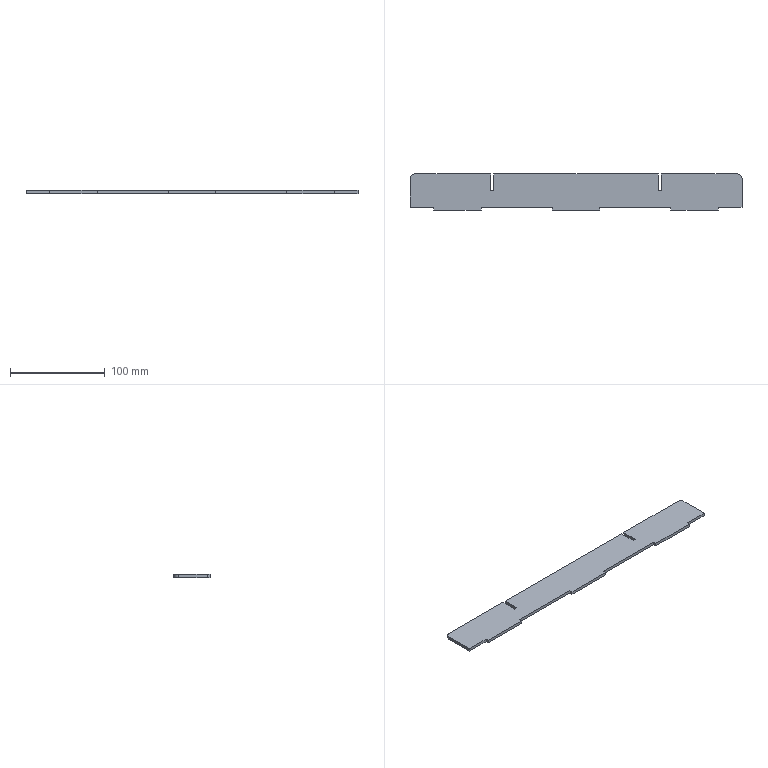Part | SolidWorks | features FlatPattern 1, SMBaseFlange 1, SheetMetal 1 | 1 solid | 28 faces | box 350 x 38 x 3.2 mm | volume 40245 mm3 | plane 26 | cylinder 2 | commonest cylinder face diameters 10 x2
STEP:
#1=CARTESIAN_POINT('',(179.887,-198.,0.));
#2=VERTEX_POINT('',#1);
#3=CARTESIAN_POINT('',(179.887,-168.,0.));
#4=VERTEX_POINT('',#3);
#5=CARTESIAN_POINT('',(179.887,-198.,0.));
#6=DIRECTION('',(0.,1.,0.));
#7=VECTOR('',#6,1000.);
#8=LINE('',#5,#7);
#9=EDGE_CURVE('',#2,#4,#8,.T.);
#10=ORIENTED_EDGE('',*,*,#9,.F.);
#11=CARTESIAN_POINT('',(179.887,-198.,-3.2));
#12=VERTEX_POINT('',#11);
#13=CARTESIAN_POINT('',(179.887,-198.,-3.2));
#14=DIRECTION('',(0.,0.,1.));
#15=VECTOR('',#14,1000.);
#16=LINE('',#13,#15);
#17=EDGE_CURVE('',#12,#2,#16,.T.);
#18=ORIENTED_EDGE('',*,*,#17,.F.);
#19=CARTESIAN_POINT('',(179.887,-168.,-3.2));
#20=VERTEX_POINT('',#19);
#21=CARTESIAN_POINT('',(179.887,-198.,-3.2));
#22=DIRECTION('',(0.,1.,0.));
#23=VECTOR('',#22,1000.);
#24=LINE('',#21,#23);
#25=EDGE_CURVE('',#12,#20,#24,.T.);
#26=ORIENTED_EDGE('',*,*,#25,.T.);
#27=CARTESIAN_POINT('',(179.887,-168.,-3.2));
#28=DIRECTION('',(0.,0.,1.));
#29=VECTOR('',#28,1000.);
#30=LINE('',#27,#29);
#31=EDGE_CURVE('',#20,#4,#30,.T.);
#32=ORIENTED_EDGE('',*,*,#31,.T.);
#33=EDGE_LOOP('',(#10,#18,#26,#32));
#34=FACE_OUTER_BOUND('',#33,.T.);
#35=CARTESIAN_POINT('',(179.887,-198.,-3.2));
#36=DIRECTION('',(1.,0.,0.));
#37=DIRECTION('',(0.,0.,-1.));
#38=AXIS2_PLACEMENT_3D('',#35,#36,#37);
#39=PLANE('',#38);
#40=ADVANCED_FACE('',(#34),#39,.T.);
#41=CARTESIAN_POINT('',(154.887,-198.,0.));
#42=VERTEX_POINT('',#41);
#43=CARTESIAN_POINT('',(179.887,-198.,0.));
#44=DIRECTION('',(1.,0.,0.));
#45=VECTOR('',#44,1000.);
#46=LINE('',#43,#45);
#47=EDGE_CURVE('',#42,#2,#46,.T.);
#48=ORIENTED_EDGE('',*,*,#47,.F.);
#49=CARTESIAN_POINT('',(154.887,-198.,-3.2));
#50=VERTEX_POINT('',#49);
#51=CARTESIAN_POINT('',(154.887,-198.,-3.2));
#52=DIRECTION('',(0.,0.,1.));
#53=VECTOR('',#52,1000.);
#54=LINE('',#51,#53);
#55=EDGE_CURVE('',#50,#42,#54,.T.);
#56=ORIENTED_EDGE('',*,*,#55,.F.);
#57=CARTESIAN_POINT('',(179.887,-198.,-3.2));
#58=DIRECTION('',(1.,0.,0.));
#59=VECTOR('',#58,1000.);
#60=LINE('',#57,#59);
#61=EDGE_CURVE('',#50,#12,#60,.T.);
#62=ORIENTED_EDGE('',*,*,#61,.T.);
#63=ORIENTED_EDGE('',*,*,#17,.T.);
#64=EDGE_LOOP('',(#48,#56,#62,#63));
#65=FACE_OUTER_BOUND('',#64,.T.);
#66=CARTESIAN_POINT('',(179.887,-198.,-3.2));
#67=DIRECTION('',(0.,-1.,0.));
#68=DIRECTION('',(0.,0.,-1.));
#69=AXIS2_PLACEMENT_3D('',#66,#67,#68);
#70=PLANE('',#69);
#71=ADVANCED_FACE('',(#65),#70,.T.);
#72=CARTESIAN_POINT('',(154.887,-201.,0.));
#73=VERTEX_POINT('',#72);
#74=CARTESIAN_POINT('',(154.887,-198.,0.));
#75=DIRECTION('',(0.,1.,0.));
#76=VECTOR('',#75,1000.);
#77=LINE('',#74,#76);
#78=EDGE_CURVE('',#73,#42,#77,.T.);
#79=ORIENTED_EDGE('',*,*,#78,.F.);
#80=CARTESIAN_POINT('',(154.887,-201.,-3.2));
#81=VERTEX_POINT('',#80);
#82=CARTESIAN_POINT('',(154.887,-201.,-3.2));
#83=DIRECTION('',(0.,0.,1.));
#84=VECTOR('',#83,1000.);
#85=LINE('',#82,#84);
#86=EDGE_CURVE('',#81,#73,#85,.T.);
#87=ORIENTED_EDGE('',*,*,#86,.F.);
#88=CARTESIAN_POINT('',(154.887,-198.,-3.2));
#89=DIRECTION('',(0.,1.,0.));
#90=VECTOR('',#89,1000.);
#91=LINE('',#88,#90);
#92=EDGE_CURVE('',#81,#50,#91,.T.);
#93=ORIENTED_EDGE('',*,*,#92,.T.);
#94=ORIENTED_EDGE('',*,*,#55,.T.);
#95=EDGE_LOOP('',(#79,#87,#93,#94));
#96=FACE_OUTER_BOUND('',#95,.T.);
#97=CARTESIAN_POINT('',(154.887,-198.,-3.2));
#98=DIRECTION('',(1.,0.,0.));
#99=DIRECTION('',(0.,0.,-1.));
#100=AXIS2_PLACEMENT_3D('',#97,#98,#99);
#101=PLANE('',#100);
#102=ADVANCED_FACE('',(#96),#101,.T.);
#103=CARTESIAN_POINT('',(104.887,-201.,0.));
#104=VERTEX_POINT('',#103);
#105=CARTESIAN_POINT('',(154.887,-201.,0.));
#106=DIRECTION('',(1.,0.,0.));
#107=VECTOR('',#106,1000.);
#108=LINE('',#105,#107);
#109=EDGE_CURVE('',#104,#73,#108,.T.);
#110=ORIENTED_EDGE('',*,*,#109,.F.);
#111=CARTESIAN_POINT('',(104.887,-201.,-3.2));
#112=VERTEX_POINT('',#111);
#113=CARTESIAN_POINT('',(104.887,-201.,-3.2));
#114=DIRECTION('',(0.,0.,1.));
#115=VECTOR('',#114,1000.);
#116=LINE('',#113,#115);
#117=EDGE_CURVE('',#112,#104,#116,.T.);
#118=ORIENTED_EDGE('',*,*,#117,.F.);
#119=CARTESIAN_POINT('',(154.887,-201.,-3.2));
#120=DIRECTION('',(1.,0.,0.));
#121=VECTOR('',#120,1000.);
#122=LINE('',#119,#121);
#123=EDGE_CURVE('',#112,#81,#122,.T.);
#124=ORIENTED_EDGE('',*,*,#123,.T.);
#125=ORIENTED_EDGE('',*,*,#86,.T.);
#126=EDGE_LOOP('',(#110,#118,#124,#125));
#127=FACE_OUTER_BOUND('',#126,.T.);
#128=CARTESIAN_POINT('',(154.887,-201.,-3.2));
#129=DIRECTION('',(0.,-1.,0.));
#130=DIRECTION('',(1.,0.,0.));
#131=AXIS2_PLACEMENT_3D('',#128,#129,#130);
#132=PLANE('',#131);
#133=ADVANCED_FACE('',(#127),#132,.T.);
#134=CARTESIAN_POINT('',(104.887,-198.,0.));
#135=VERTEX_POINT('',#134);
#136=CARTESIAN_POINT('',(104.887,-201.,0.));
#137=DIRECTION('',(0.,-1.,0.));
#138=VECTOR('',#137,1000.);
#139=LINE('',#136,#138);
#140=EDGE_CURVE('',#135,#104,#139,.T.);
#141=ORIENTED_EDGE('',*,*,#140,.F.);
#142=CARTESIAN_POINT('',(104.887,-198.,-3.2));
#143=VERTEX_POINT('',#142);
#144=CARTESIAN_POINT('',(104.887,-198.,-3.2));
#145=DIRECTION('',(0.,0.,1.));
#146=VECTOR('',#145,1000.);
#147=LINE('',#144,#146);
#148=EDGE_CURVE('',#143,#135,#147,.T.);
#149=ORIENTED_EDGE('',*,*,#148,.F.);
#150=CARTESIAN_POINT('',(104.887,-201.,-3.2));
#151=DIRECTION('',(0.,-1.,0.));
#152=VECTOR('',#151,1000.);
#153=LINE('',#150,#152);
#154=EDGE_CURVE('',#143,#112,#153,.T.);
#155=ORIENTED_EDGE('',*,*,#154,.T.);
#156=ORIENTED_EDGE('',*,*,#117,.T.);
#157=EDGE_LOOP('',(#141,#149,#155,#156));
#158=FACE_OUTER_BOUND('',#157,.T.);
#159=CARTESIAN_POINT('',(104.887,-201.,-3.2));
#160=DIRECTION('',(-1.,0.,0.));
#161=DIRECTION('',(0.,-1.,0.));
#162=AXIS2_PLACEMENT_3D('',#159,#160,#161);
#163=PLANE('',#162);
#164=ADVANCED_FACE('',(#158),#163,.T.);
#165=CARTESIAN_POINT('',(29.887,-198.,0.));
#166=VERTEX_POINT('',#165);
#167=CARTESIAN_POINT('',(104.887,-198.,0.));
#168=DIRECTION('',(1.,0.,0.));
#169=VECTOR('',#168,1000.);
#170=LINE('',#167,#169);
#171=EDGE_CURVE('',#166,#135,#170,.T.);
#172=ORIENTED_EDGE('',*,*,#171,.F.);
#173=CARTESIAN_POINT('',(29.887,-198.,-3.2));
#174=VERTEX_POINT('',#173);
#175=CARTESIAN_POINT('',(29.887,-198.,-3.2));
#176=DIRECTION('',(0.,0.,1.));
#177=VECTOR('',#176,1000.);
#178=LINE('',#175,#177);
#179=EDGE_CURVE('',#174,#166,#178,.T.);
#180=ORIENTED_EDGE('',*,*,#179,.F.);
#181=CARTESIAN_POINT('',(104.887,-198.,-3.2));
#182=DIRECTION('',(1.,0.,0.));
#183=VECTOR('',#182,1000.);
#184=LINE('',#181,#183);
#185=EDGE_CURVE('',#174,#143,#184,.T.);
#186=ORIENTED_EDGE('',*,*,#185,.T.);
#187=ORIENTED_EDGE('',*,*,#148,.T.);
#188=EDGE_LOOP('',(#172,#180,#186,#187));
#189=FACE_OUTER_BOUND('',#188,.T.);
#190=CARTESIAN_POINT('',(104.887,-198.,-3.2));
#191=DIRECTION('',(0.,-1.,0.));
#192=DIRECTION('',(1.,0.,0.));
#193=AXIS2_PLACEMENT_3D('',#190,#191,#192);
#194=PLANE('',#193);
#195=ADVANCED_FACE('',(#189),#194,.T.);
#196=CARTESIAN_POINT('',(29.887,-201.,0.));
#197=VERTEX_POINT('',#196);
#198=CARTESIAN_POINT('',(29.887,-198.,0.));
#199=DIRECTION('',(0.,1.,0.));
#200=VECTOR('',#199,1000.);
#201=LINE('',#198,#200);
#202=EDGE_CURVE('',#197,#166,#201,.T.);
#203=ORIENTED_EDGE('',*,*,#202,.F.);
#204=CARTESIAN_POINT('',(29.887,-201.,-3.2));
#205=VERTEX_POINT('',#204);
#206=CARTESIAN_POINT('',(29.887,-201.,-3.2));
#207=DIRECTION('',(0.,0.,1.));
#208=VECTOR('',#207,1000.);
#209=LINE('',#206,#208);
#210=EDGE_CURVE('',#205,#197,#209,.T.);
#211=ORIENTED_EDGE('',*,*,#210,.F.);
#212=CARTESIAN_POINT('',(29.887,-198.,-3.2));
#213=DIRECTION('',(0.,1.,0.));
#214=VECTOR('',#213,1000.);
#215=LINE('',#212,#214);
#216=EDGE_CURVE('',#205,#174,#215,.T.);
#217=ORIENTED_EDGE('',*,*,#216,.T.);
#218=ORIENTED_EDGE('',*,*,#179,.T.);
#219=EDGE_LOOP('',(#203,#211,#217,#218));
#220=FACE_OUTER_BOUND('',#219,.T.);
#221=CARTESIAN_POINT('',(29.887,-198.,-3.2));
#222=DIRECTION('',(1.,0.,0.));
#223=DIRECTION('',(0.,1.,0.));
#224=AXIS2_PLACEMENT_3D('',#221,#222,#223);
#225=PLANE('',#224);
#226=ADVANCED_FACE('',(#220),#225,.T.);
#227=CARTESIAN_POINT('',(-20.113,-201.,0.));
#228=VERTEX_POINT('',#227);
#229=CARTESIAN_POINT('',(29.887,-201.,0.));
#230=DIRECTION('',(1.,0.,0.));
#231=VECTOR('',#230,1000.);
#232=LINE('',#229,#231);
#233=EDGE_CURVE('',#228,#197,#232,.T.);
#234=ORIENTED_EDGE('',*,*,#233,.F.);
#235=CARTESIAN_POINT('',(-20.113,-201.,-3.2));
#236=VERTEX_POINT('',#235);
#237=CARTESIAN_POINT('',(-20.113,-201.,-3.2));
#238=DIRECTION('',(0.,0.,1.));
#239=VECTOR('',#238,1000.);
#240=LINE('',#237,#239);
#241=EDGE_CURVE('',#236,#228,#240,.T.);
#242=ORIENTED_EDGE('',*,*,#241,.F.);
#243=CARTESIAN_POINT('',(29.887,-201.,-3.2));
#244=DIRECTION('',(1.,0.,0.));
#245=VECTOR('',#244,1000.);
#246=LINE('',#243,#245);
#247=EDGE_CURVE('',#236,#205,#246,.T.);
#248=ORIENTED_EDGE('',*,*,#247,.T.);
#249=ORIENTED_EDGE('',*,*,#210,.T.);
#250=EDGE_LOOP('',(#234,#242,#248,#249));
#251=FACE_OUTER_BOUND('',#250,.T.);
#252=CARTESIAN_POINT('',(29.887,-201.,-3.2));
#253=DIRECTION('',(0.,-1.,0.));
#254=DIRECTION('',(0.,0.,-1.));
#255=AXIS2_PLACEMENT_3D('',#252,#253,#254);
#256=PLANE('',#255);
#257=ADVANCED_FACE('',(#251),#256,.T.);
#258=CARTESIAN_POINT('',(-20.113,-198.,0.));
#259=VERTEX_POINT('',#258);
#260=CARTESIAN_POINT('',(-20.113,-201.,0.));
#261=DIRECTION('',(0.,-1.,0.));
#262=VECTOR('',#261,1000.);
#263=LINE('',#260,#262);
#264=EDGE_CURVE('',#259,#228,#263,.T.);
#265=ORIENTED_EDGE('',*,*,#264,.F.);
#266=CARTESIAN_POINT('',(-20.113,-198.,-3.2));
#267=VERTEX_POINT('',#266);
#268=CARTESIAN_POINT('',(-20.113,-198.,-3.2));
#269=DIRECTION('',(0.,0.,1.));
#270=VECTOR('',#269,1000.);
#271=LINE('',#268,#270);
#272=EDGE_CURVE('',#267,#259,#271,.T.);
#273=ORIENTED_EDGE('',*,*,#272,.F.);
#274=CARTESIAN_POINT('',(-20.113,-201.,-3.2));
#275=DIRECTION('',(0.,-1.,0.));
#276=VECTOR('',#275,1000.);
#277=LINE('',#274,#276);
#278=EDGE_CURVE('',#267,#236,#277,.T.);
#279=ORIENTED_EDGE('',*,*,#278,.T.);
#280=ORIENTED_EDGE('',*,*,#241,.T.);
#281=EDGE_LOOP('',(#265,#273,#279,#280));
#282=FACE_OUTER_BOUND('',#281,.T.);
#283=CARTESIAN_POINT('',(-20.113,-201.,-3.2));
#284=DIRECTION('',(-1.,0.,0.));
#285=DIRECTION('',(0.,0.,1.));
#286=AXIS2_PLACEMENT_3D('',#283,#284,#285);
#287=PLANE('',#286);
#288=ADVANCED_FACE('',(#282),#287,.T.);
#289=CARTESIAN_POINT('',(-95.113,-198.,0.));
#290=VERTEX_POINT('',#289);
#291=CARTESIAN_POINT('',(-20.113,-198.,0.));
#292=DIRECTION('',(1.,0.,0.));
#293=VECTOR('',#292,1000.);
#294=LINE('',#291,#293);
#295=EDGE_CURVE('',#290,#259,#294,.T.);
#296=ORIENTED_EDGE('',*,*,#295,.F.);
#297=CARTESIAN_POINT('',(-95.113,-198.,-3.2));
#298=VERTEX_POINT('',#297);
#299=CARTESIAN_POINT('',(-95.113,-198.,-3.2));
#300=DIRECTION('',(0.,0.,1.));
#301=VECTOR('',#300,1000.);
#302=LINE('',#299,#301);
#303=EDGE_CURVE('',#298,#290,#302,.T.);
#304=ORIENTED_EDGE('',*,*,#303,.F.);
#305=CARTESIAN_POINT('',(-20.113,-198.,-3.2));
#306=DIRECTION('',(1.,0.,0.));
#307=VECTOR('',#306,1000.);
#308=LINE('',#305,#307);
#309=EDGE_CURVE('',#298,#267,#308,.T.);
#310=ORIENTED_EDGE('',*,*,#309,.T.);
#311=ORIENTED_EDGE('',*,*,#272,.T.);
#312=EDGE_LOOP('',(#296,#304,#310,#311));
#313=FACE_OUTER_BOUND('',#312,.T.);
#314=CARTESIAN_POINT('',(-20.113,-198.,-3.2));
#315=DIRECTION('',(0.,-1.,0.));
#316=DIRECTION('',(0.,0.,-1.));
#317=AXIS2_PLACEMENT_3D('',#314,#315,#316);
#318=PLANE('',#317);
#319=ADVANCED_FACE('',(#313),#318,.T.);
#320=CARTESIAN_POINT('',(-95.113,-201.,0.));
#321=VERTEX_POINT('',#320);
#322=CARTESIAN_POINT('',(-95.113,-201.,0.));
#323=DIRECTION('',(0.,1.,0.));
#324=VECTOR('',#323,1000.);
#325=LINE('',#322,#324);
#326=EDGE_CURVE('',#321,#290,#325,.T.);
#327=ORIENTED_EDGE('',*,*,#326,.F.);
#328=CARTESIAN_POINT('',(-95.113,-201.,-3.2));
#329=VERTEX_POINT('',#328);
#330=CARTESIAN_POINT('',(-95.113,-201.,-3.2));
#331=DIRECTION('',(0.,0.,1.));
#332=VECTOR('',#331,1000.);
#333=LINE('',#330,#332);
#334=EDGE_CURVE('',#329,#321,#333,.T.);
#335=ORIENTED_EDGE('',*,*,#334,.F.);
#336=CARTESIAN_POINT('',(-95.113,-201.,-3.2));
#337=DIRECTION('',(0.,1.,0.));
#338=VECTOR('',#337,1000.);
#339=LINE('',#336,#338);
#340=EDGE_CURVE('',#329,#298,#339,.T.);
#341=ORIENTED_EDGE('',*,*,#340,.T.);
#342=ORIENTED_EDGE('',*,*,#303,.T.);
#343=EDGE_LOOP('',(#327,#335,#341,#342));
#344=FACE_OUTER_BOUND('',#343,.T.);
#345=CARTESIAN_POINT('',(-95.113,-201.,-3.2));
#346=DIRECTION('',(1.,0.,0.));
#347=DIRECTION('',(0.,0.,-1.));
#348=AXIS2_PLACEMENT_3D('',#345,#346,#347);
#349=PLANE('',#348);
#350=ADVANCED_FACE('',(#344),#349,.T.);
#351=CARTESIAN_POINT('',(-145.113,-201.,0.));
#352=VERTEX_POINT('',#351);
#353=CARTESIAN_POINT('',(-145.113,-201.,0.));
#354=DIRECTION('',(1.,0.,0.));
#355=VECTOR('',#354,1000.);
#356=LINE('',#353,#355);
#357=EDGE_CURVE('',#352,#321,#356,.T.);
#358=ORIENTED_EDGE('',*,*,#357,.F.);
#359=CARTESIAN_POINT('',(-145.113,-201.,-3.2));
#360=VERTEX_POINT('',#359);
#361=CARTESIAN_POINT('',(-145.113,-201.,-3.2));
#362=DIRECTION('',(0.,0.,1.));
#363=VECTOR('',#362,1000.);
#364=LINE('',#361,#363);
#365=EDGE_CURVE('',#360,#352,#364,.T.);
#366=ORIENTED_EDGE('',*,*,#365,.F.);
#367=CARTESIAN_POINT('',(-145.113,-201.,-3.2));
#368=DIRECTION('',(1.,0.,0.));
#369=VECTOR('',#368,1000.);
#370=LINE('',#367,#369);
#371=EDGE_CURVE('',#360,#329,#370,.T.);
#372=ORIENTED_EDGE('',*,*,#371,.T.);
#373=ORIENTED_EDGE('',*,*,#334,.T.);
#374=EDGE_LOOP('',(#358,#366,#372,#373));
#375=FACE_OUTER_BOUND('',#374,.T.);
#376=CARTESIAN_POINT('',(-145.113,-201.,-3.2));
#377=DIRECTION('',(0.,-1.,0.));
#378=DIRECTION('',(1.,0.,0.));
#379=AXIS2_PLACEMENT_3D('',#376,#377,#378);
#380=PLANE('',#379);
#381=ADVANCED_FACE('',(#375),#380,.T.);
#382=CARTESIAN_POINT('',(-145.113,-198.,0.));
#383=VERTEX_POINT('',#382);
#384=CARTESIAN_POINT('',(-145.113,-198.,0.));
#385=DIRECTION('',(0.,-1.,0.));
#386=VECTOR('',#385,1000.);
#387=LINE('',#384,#386);
#388=EDGE_CURVE('',#383,#352,#387,.T.);
#389=ORIENTED_EDGE('',*,*,#388,.F.);
#390=CARTESIAN_POINT('',(-145.113,-198.,-3.2));
#391=VERTEX_POINT('',#390);
#392=CARTESIAN_POINT('',(-145.113,-198.,-3.2));
#393=DIRECTION('',(0.,0.,1.));
#394=VECTOR('',#393,1000.);
#395=LINE('',#392,#394);
#396=EDGE_CURVE('',#391,#383,#395,.T.);
#397=ORIENTED_EDGE('',*,*,#396,.F.);
#398=CARTESIAN_POINT('',(-145.113,-198.,-3.2));
#399=DIRECTION('',(0.,-1.,0.));
#400=VECTOR('',#399,1000.);
#401=LINE('',#398,#400);
#402=EDGE_CURVE('',#391,#360,#401,.T.);
#403=ORIENTED_EDGE('',*,*,#402,.T.);
#404=ORIENTED_EDGE('',*,*,#365,.T.);
#405=EDGE_LOOP('',(#389,#397,#403,#404));
#406=FACE_OUTER_BOUND('',#405,.T.);
#407=CARTESIAN_POINT('',(-145.113,-198.,-3.2));
#408=DIRECTION('',(-1.,0.,0.));
#409=DIRECTION('',(0.,0.,1.));
#410=AXIS2_PLACEMENT_3D('',#407,#408,#409);
#411=PLANE('',#410);
#412=ADVANCED_FACE('',(#406),#411,.T.);
#413=CARTESIAN_POINT('',(-170.113,-198.,0.));
#414=VERTEX_POINT('',#413);
#415=CARTESIAN_POINT('',(-145.113,-198.,0.));
#416=DIRECTION('',(1.,0.,0.));
#417=VECTOR('',#416,1000.);
#418=LINE('',#415,#417);
#419=EDGE_CURVE('',#414,#383,#418,.T.);
#420=ORIENTED_EDGE('',*,*,#419,.F.);
#421=CARTESIAN_POINT('',(-170.113,-198.,-3.2));
#422=VERTEX_POINT('',#421);
#423=CARTESIAN_POINT('',(-170.113,-198.,-3.2));
#424=DIRECTION('',(0.,0.,1.));
#425=VECTOR('',#424,1000.);
#426=LINE('',#423,#425);
#427=EDGE_CURVE('',#422,#414,#426,.T.);
#428=ORIENTED_EDGE('',*,*,#427,.F.);
#429=CARTESIAN_POINT('',(-145.113,-198.,-3.2));
#430=DIRECTION('',(1.,0.,0.));
#431=VECTOR('',#430,1000.);
#432=LINE('',#429,#431);
#433=EDGE_CURVE('',#422,#391,#432,.T.);
#434=ORIENTED_EDGE('',*,*,#433,.T.);
#435=ORIENTED_EDGE('',*,*,#396,.T.);
#436=EDGE_LOOP('',(#420,#428,#434,#435));
#437=FACE_OUTER_BOUND('',#436,.T.);
#438=CARTESIAN_POINT('',(-145.113,-198.,-3.2));
#439=DIRECTION('',(0.,-1.,0.));
#440=DIRECTION('',(1.,0.,0.));
#441=AXIS2_PLACEMENT_3D('',#438,#439,#440);
#442=PLANE('',#441);
#443=ADVANCED_FACE('',(#437),#442,.T.);
#444=CARTESIAN_POINT('',(-170.113,-168.,0.));
#445=VERTEX_POINT('',#444);
#446=CARTESIAN_POINT('',(-170.113,-198.,0.));
#447=DIRECTION('',(0.,-1.,0.));
#448=VECTOR('',#447,1000.);
#449=LINE('',#446,#448);
#450=EDGE_CURVE('',#445,#414,#449,.T.);
#451=ORIENTED_EDGE('',*,*,#450,.F.);
#452=CARTESIAN_POINT('',(-170.113,-168.,-3.2));
#453=VERTEX_POINT('',#452);
#454=CARTESIAN_POINT('',(-170.113,-168.,-3.2));
#455=DIRECTION('',(0.,0.,1.));
#456=VECTOR('',#455,1000.);
#457=LINE('',#454,#456);
#458=EDGE_CURVE('',#453,#445,#457,.T.);
#459=ORIENTED_EDGE('',*,*,#458,.F.);
#460=CARTESIAN_POINT('',(-170.113,-198.,-3.2));
#461=DIRECTION('',(0.,-1.,0.));
#462=VECTOR('',#461,1000.);
#463=LINE('',#460,#462);
#464=EDGE_CURVE('',#453,#422,#463,.T.);
#465=ORIENTED_EDGE('',*,*,#464,.T.);
#466=ORIENTED_EDGE('',*,*,#427,.T.);
#467=EDGE_LOOP('',(#451,#459,#465,#466));
#468=FACE_OUTER_BOUND('',#467,.T.);
#469=CARTESIAN_POINT('',(-170.113,-198.,-3.2));
#470=DIRECTION('',(-1.,0.,0.));
#471=DIRECTION('',(0.,0.,1.));
#472=AXIS2_PLACEMENT_3D('',#469,#470,#471);
#473=PLANE('',#472);
#474=ADVANCED_FACE('',(#468),#473,.T.);
#475=CARTESIAN_POINT('',(-165.113,-163.,0.));
#476=VERTEX_POINT('',#475);
#477=CARTESIAN_POINT('',(-165.113,-168.,0.));
#478=DIRECTION('',(0.,0.,1.));
#479=DIRECTION('',(1.,0.,0.));
#480=AXIS2_PLACEMENT_3D('',#477,#478,#479);
#481=CIRCLE('',#480,5.);
#482=EDGE_CURVE('',#476,#445,#481,.T.);
#483=ORIENTED_EDGE('',*,*,#482,.F.);
#484=CARTESIAN_POINT('',(-165.113,-163.,-3.2));
#485=VERTEX_POINT('',#484);
#486=CARTESIAN_POINT('',(-165.113,-163.,-3.2));
#487=DIRECTION('',(0.,0.,1.));
#488=VECTOR('',#487,1000.);
#489=LINE('',#486,#488);
#490=EDGE_CURVE('',#485,#476,#489,.T.);
#491=ORIENTED_EDGE('',*,*,#490,.F.);
#492=CARTESIAN_POINT('',(-165.113,-168.,-3.2));
#493=DIRECTION('',(0.,0.,1.));
#494=DIRECTION('',(1.,0.,0.));
#495=AXIS2_PLACEMENT_3D('',#492,#493,#494);
#496=CIRCLE('',#495,5.);
#497=EDGE_CURVE('',#485,#453,#496,.T.);
#498=ORIENTED_EDGE('',*,*,#497,.T.);
#499=ORIENTED_EDGE('',*,*,#458,.T.);
#500=EDGE_LOOP('',(#483,#491,#498,#499));
#501=FACE_OUTER_BOUND('',#500,.T.);
#502=CARTESIAN_POINT('',(-165.113,-168.,-3.2));
#503=DIRECTION('',(0.,0.,1.));
#504=DIRECTION('',(1.,0.,0.));
#505=AXIS2_PLACEMENT_3D('',#502,#503,#504);
#506=CYLINDRICAL_SURFACE('',#505,5.);
#507=ADVANCED_FACE('',(#501),#506,.T.);
#508=CARTESIAN_POINT('',(-85.113,-163.,0.));
#509=VERTEX_POINT('',#508);
#510=CARTESIAN_POINT('',(-85.113,-163.,0.));
#511=DIRECTION('',(-1.,0.,0.));
#512=VECTOR('',#511,1000.);
#513=LINE('',#510,#512);
#514=EDGE_CURVE('',#509,#476,#513,.T.);
#515=ORIENTED_EDGE('',*,*,#514,.F.);
#516=CARTESIAN_POINT('',(-85.113,-163.,-3.2));
#517=VERTEX_POINT('',#516);
#518=CARTESIAN_POINT('',(-85.113,-163.,-3.2));
#519=DIRECTION('',(0.,0.,1.));
#520=VECTOR('',#519,1000.);
#521=LINE('',#518,#520);
#522=EDGE_CURVE('',#517,#509,#521,.T.);
#523=ORIENTED_EDGE('',*,*,#522,.F.);
#524=CARTESIAN_POINT('',(-85.113,-163.,-3.2));
#525=DIRECTION('',(-1.,0.,0.));
#526=VECTOR('',#525,1000.);
#527=LINE('',#524,#526);
#528=EDGE_CURVE('',#517,#485,#527,.T.);
#529=ORIENTED_EDGE('',*,*,#528,.T.);
#530=ORIENTED_EDGE('',*,*,#490,.T.);
#531=EDGE_LOOP('',(#515,#523,#529,#530));
#532=FACE_OUTER_BOUND('',#531,.T.);
#533=CARTESIAN_POINT('',(-85.113,-163.,-3.2));
#534=DIRECTION('',(0.,1.,0.));
#535=DIRECTION('',(-1.,0.,0.));
#536=AXIS2_PLACEMENT_3D('',#533,#534,#535);
#537=PLANE('',#536);
#538=ADVANCED_FACE('',(#532),#537,.T.);
#539=CARTESIAN_POINT('',(-85.113,-180.6,0.));
#540=VERTEX_POINT('',#539);
#541=CARTESIAN_POINT('',(-85.113,-180.6,0.));
#542=DIRECTION('',(0.,1.,0.));
#543=VECTOR('',#542,1000.);
#544=LINE('',#541,#543);
#545=EDGE_CURVE('',#540,#509,#544,.T.);
#546=ORIENTED_EDGE('',*,*,#545,.F.);
#547=CARTESIAN_POINT('',(-85.113,-180.6,-3.2));
#548=VERTEX_POINT('',#547);
#549=CARTESIAN_POINT('',(-85.113,-180.6,-3.2));
#550=DIRECTION('',(0.,0.,1.));
#551=VECTOR('',#550,1000.);
#552=LINE('',#549,#551);
#553=EDGE_CURVE('',#548,#540,#552,.T.);
#554=ORIENTED_EDGE('',*,*,#553,.F.);
#555=CARTESIAN_POINT('',(-85.113,-180.6,-3.2));
#556=DIRECTION('',(0.,1.,0.));
#557=VECTOR('',#556,1000.);
#558=LINE('',#555,#557);
#559=EDGE_CURVE('',#548,#517,#558,.T.);
#560=ORIENTED_EDGE('',*,*,#559,.T.);
#561=ORIENTED_EDGE('',*,*,#522,.T.);
#562=EDGE_LOOP('',(#546,#554,#560,#561));
#563=FACE_OUTER_BOUND('',#562,.T.);
#564=CARTESIAN_POINT('',(-85.113,-180.6,-3.2));
#565=DIRECTION('',(1.,0.,0.));
#566=DIRECTION('',(0.,1.,0.));
#567=AXIS2_PLACEMENT_3D('',#564,#565,#566);
#568=PLANE('',#567);
#569=ADVANCED_FACE('',(#563),#568,.T.);
#570=CARTESIAN_POINT('',(-81.913,-180.6,0.));
#571=VERTEX_POINT('',#570);
#572=CARTESIAN_POINT('',(-81.913,-180.6,0.));
#573=DIRECTION('',(-1.,0.,0.));
#574=VECTOR('',#573,1000.);
#575=LINE('',#572,#574);
#576=EDGE_CURVE('',#571,#540,#575,.T.);
#577=ORIENTED_EDGE('',*,*,#576,.F.);
#578=CARTESIAN_POINT('',(-81.913,-180.6,-3.2));
#579=VERTEX_POINT('',#578);
#580=CARTESIAN_POINT('',(-81.913,-180.6,-3.2));
#581=DIRECTION('',(0.,0.,1.));
#582=VECTOR('',#581,1000.);
#583=LINE('',#580,#582);
#584=EDGE_CURVE('',#579,#571,#583,.T.);
#585=ORIENTED_EDGE('',*,*,#584,.F.);
#586=CARTESIAN_POINT('',(-81.913,-180.6,-3.2));
#587=DIRECTION('',(-1.,0.,0.));
#588=VECTOR('',#587,1000.);
#589=LINE('',#586,#588);
#590=EDGE_CURVE('',#579,#548,#589,.T.);
#591=ORIENTED_EDGE('',*,*,#590,.T.);
#592=ORIENTED_EDGE('',*,*,#553,.T.);
#593=EDGE_LOOP('',(#577,#585,#591,#592));
#594=FACE_OUTER_BOUND('',#593,.T.);
#595=CARTESIAN_POINT('',(-81.913,-180.6,-3.2));
#596=DIRECTION('',(0.,1.,0.));
#597=DIRECTION('',(0.,0.,1.));
#598=AXIS2_PLACEMENT_3D('',#595,#596,#597);
#599=PLANE('',#598);
#600=ADVANCED_FACE('',(#594),#599,.T.);
#601=CARTESIAN_POINT('',(-81.913,-163.,0.));
#602=VERTEX_POINT('',#601);
#603=CARTESIAN_POINT('',(-81.913,-163.,0.));
#604=DIRECTION('',(0.,-1.,0.));
#605=VECTOR('',#604,1000.);
#606=LINE('',#603,#605);
#607=EDGE_CURVE('',#602,#571,#606,.T.);
#608=ORIENTED_EDGE('',*,*,#607,.F.);
#609=CARTESIAN_POINT('',(-81.913,-163.,-3.2));
#610=VERTEX_POINT('',#609);
#611=CARTESIAN_POINT('',(-81.913,-163.,-3.2));
#612=DIRECTION('',(0.,0.,1.));
#613=VECTOR('',#612,1000.);
#614=LINE('',#611,#613);
#615=EDGE_CURVE('',#610,#602,#614,.T.);
#616=ORIENTED_EDGE('',*,*,#615,.F.);
#617=CARTESIAN_POINT('',(-81.913,-163.,-3.2));
#618=DIRECTION('',(0.,-1.,0.));
#619=VECTOR('',#618,1000.);
#620=LINE('',#617,#619);
#621=EDGE_CURVE('',#610,#579,#620,.T.);
#622=ORIENTED_EDGE('',*,*,#621,.T.);
#623=ORIENTED_EDGE('',*,*,#584,.T.);
#624=EDGE_LOOP('',(#608,#616,#622,#623));
#625=FACE_OUTER_BOUND('',#624,.T.);
#626=CARTESIAN_POINT('',(-81.913,-163.,-3.2));
#627=DIRECTION('',(-1.,0.,0.));
#628=DIRECTION('',(0.,-1.,0.));
#629=AXIS2_PLACEMENT_3D('',#626,#627,#628);
#630=PLANE('',#629);
#631=ADVANCED_FACE('',(#625),#630,.T.);
#632=CARTESIAN_POINT('',(91.687,-163.,0.));
#633=VERTEX_POINT('',#632);
#634=CARTESIAN_POINT('',(91.687,-163.,0.));
#635=DIRECTION('',(-1.,0.,0.));
#636=VECTOR('',#635,1000.);
#637=LINE('',#634,#636);
#638=EDGE_CURVE('',#633,#602,#637,.T.);
#639=ORIENTED_EDGE('',*,*,#638,.F.);
#640=CARTESIAN_POINT('',(91.687,-163.,-3.2));
#641=VERTEX_POINT('',#640);
#642=CARTESIAN_POINT('',(91.687,-163.,-3.2));
#643=DIRECTION('',(0.,0.,1.));
#644=VECTOR('',#643,1000.);
#645=LINE('',#642,#644);
#646=EDGE_CURVE('',#641,#633,#645,.T.);
#647=ORIENTED_EDGE('',*,*,#646,.F.);
#648=CARTESIAN_POINT('',(91.687,-163.,-3.2));
#649=DIRECTION('',(-1.,0.,0.));
#650=VECTOR('',#649,1000.);
#651=LINE('',#648,#650);
#652=EDGE_CURVE('',#641,#610,#651,.T.);
#653=ORIENTED_EDGE('',*,*,#652,.T.);
#654=ORIENTED_EDGE('',*,*,#615,.T.);
#655=EDGE_LOOP('',(#639,#647,#653,#654));
#656=FACE_OUTER_BOUND('',#655,.T.);
#657=CARTESIAN_POINT('',(91.687,-163.,-3.2));
#658=DIRECTION('',(0.,1.,0.));
#659=DIRECTION('',(-1.,0.,0.));
#660=AXIS2_PLACEMENT_3D('',#657,#658,#659);
#661=PLANE('',#660);
#662=ADVANCED_FACE('',(#656),#661,.T.);
#663=CARTESIAN_POINT('',(91.687,-180.6,0.));
#664=VERTEX_POINT('',#663);
#665=CARTESIAN_POINT('',(91.687,-180.6,0.));
#666=DIRECTION('',(0.,1.,0.));
#667=VECTOR('',#666,1000.);
#668=LINE('',#665,#667);
#669=EDGE_CURVE('',#664,#633,#668,.T.);
#670=ORIENTED_EDGE('',*,*,#669,.F.);
#671=CARTESIAN_POINT('',(91.687,-180.6,-3.2));
#672=VERTEX_POINT('',#671);
#673=CARTESIAN_POINT('',(91.687,-180.6,-3.2));
#674=DIRECTION('',(0.,0.,1.));
#675=VECTOR('',#674,1000.);
#676=LINE('',#673,#675);
#677=EDGE_CURVE('',#672,#664,#676,.T.);
#678=ORIENTED_EDGE('',*,*,#677,.F.);
#679=CARTESIAN_POINT('',(91.687,-180.6,-3.2));
#680=DIRECTION('',(0.,1.,0.));
#681=VECTOR('',#680,1000.);
#682=LINE('',#679,#681);
#683=EDGE_CURVE('',#672,#641,#682,.T.);
#684=ORIENTED_EDGE('',*,*,#683,.T.);
#685=ORIENTED_EDGE('',*,*,#646,.T.);
#686=EDGE_LOOP('',(#670,#678,#684,#685));
#687=FACE_OUTER_BOUND('',#686,.T.);
#688=CARTESIAN_POINT('',(91.687,-180.6,-3.2));
#689=DIRECTION('',(1.,0.,0.));
#690=DIRECTION('',(0.,1.,0.));
#691=AXIS2_PLACEMENT_3D('',#688,#689,#690);
#692=PLANE('',#691);
#693=ADVANCED_FACE('',(#687),#692,.T.);
#694=CARTESIAN_POINT('',(94.887,-180.6,0.));
#695=VERTEX_POINT('',#694);
#696=CARTESIAN_POINT('',(94.887,-180.6,0.));
#697=DIRECTION('',(-1.,0.,0.));
#698=VECTOR('',#697,1000.);
#699=LINE('',#696,#698);
#700=EDGE_CURVE('',#695,#664,#699,.T.);
#701=ORIENTED_EDGE('',*,*,#700,.F.);
#702=CARTESIAN_POINT('',(94.887,-180.6,-3.2));
#703=VERTEX_POINT('',#702);
#704=CARTESIAN_POINT('',(94.887,-180.6,-3.2));
#705=DIRECTION('',(0.,0.,1.));
#706=VECTOR('',#705,1000.);
#707=LINE('',#704,#706);
#708=EDGE_CURVE('',#703,#695,#707,.T.);
#709=ORIENTED_EDGE('',*,*,#708,.F.);
#710=CARTESIAN_POINT('',(94.887,-180.6,-3.2));
#711=DIRECTION('',(-1.,0.,0.));
#712=VECTOR('',#711,1000.);
#713=LINE('',#710,#712);
#714=EDGE_CURVE('',#703,#672,#713,.T.);
#715=ORIENTED_EDGE('',*,*,#714,.T.);
#716=ORIENTED_EDGE('',*,*,#677,.T.);
#717=EDGE_LOOP('',(#701,#709,#715,#716));
#718=FACE_OUTER_BOUND('',#717,.T.);
#719=CARTESIAN_POINT('',(94.887,-180.6,-3.2));
#720=DIRECTION('',(0.,1.,0.));
#721=DIRECTION('',(0.,0.,1.));
#722=AXIS2_PLACEMENT_3D('',#719,#720,#721);
#723=PLANE('',#722);
#724=ADVANCED_FACE('',(#718),#723,.T.);
#725=CARTESIAN_POINT('',(94.887,-163.,0.));
#726=VERTEX_POINT('',#725);
#727=CARTESIAN_POINT('',(94.887,-163.,0.));
#728=DIRECTION('',(0.,-1.,0.));
#729=VECTOR('',#728,1000.);
#730=LINE('',#727,#729);
#731=EDGE_CURVE('',#726,#695,#730,.T.);
#732=ORIENTED_EDGE('',*,*,#731,.F.);
#733=CARTESIAN_POINT('',(94.887,-163.,-3.2));
#734=VERTEX_POINT('',#733);
#735=CARTESIAN_POINT('',(94.887,-163.,-3.2));
#736=DIRECTION('',(0.,0.,1.));
#737=VECTOR('',#736,1000.);
#738=LINE('',#735,#737);
#739=EDGE_CURVE('',#734,#726,#738,.T.);
#740=ORIENTED_EDGE('',*,*,#739,.F.);
#741=CARTESIAN_POINT('',(94.887,-163.,-3.2));
#742=DIRECTION('',(0.,-1.,0.));
#743=VECTOR('',#742,1000.);
#744=LINE('',#741,#743);
#745=EDGE_CURVE('',#734,#703,#744,.T.);
#746=ORIENTED_EDGE('',*,*,#745,.T.);
#747=ORIENTED_EDGE('',*,*,#708,.T.);
#748=EDGE_LOOP('',(#732,#740,#746,#747));
#749=FACE_OUTER_BOUND('',#748,.T.);
#750=CARTESIAN_POINT('',(94.887,-163.,-3.2));
#751=DIRECTION('',(-1.,0.,0.));
#752=DIRECTION('',(0.,-1.,0.));
#753=AXIS2_PLACEMENT_3D('',#750,#751,#752);
#754=PLANE('',#753);
#755=ADVANCED_FACE('',(#749),#754,.T.);
#756=CARTESIAN_POINT('',(174.887,-163.,0.));
#757=VERTEX_POINT('',#756);
#758=CARTESIAN_POINT('',(174.887,-163.,0.));
#759=DIRECTION('',(-1.,0.,0.));
#760=VECTOR('',#759,1000.);
#761=LINE('',#758,#760);
#762=EDGE_CURVE('',#757,#726,#761,.T.);
#763=ORIENTED_EDGE('',*,*,#762,.F.);
#764=CARTESIAN_POINT('',(174.887,-163.,-3.2));
#765=VERTEX_POINT('',#764);
#766=CARTESIAN_POINT('',(174.887,-163.,-3.2));
#767=DIRECTION('',(0.,0.,1.));
#768=VECTOR('',#767,1000.);
#769=LINE('',#766,#768);
#770=EDGE_CURVE('',#765,#757,#769,.T.);
#771=ORIENTED_EDGE('',*,*,#770,.F.);
#772=CARTESIAN_POINT('',(174.887,-163.,-3.2));
#773=DIRECTION('',(-1.,0.,0.));
#774=VECTOR('',#773,1000.);
#775=LINE('',#772,#774);
#776=EDGE_CURVE('',#765,#734,#775,.T.);
#777=ORIENTED_EDGE('',*,*,#776,.T.);
#778=ORIENTED_EDGE('',*,*,#739,.T.);
#779=EDGE_LOOP('',(#763,#771,#777,#778));
#780=FACE_OUTER_BOUND('',#779,.T.);
#781=CARTESIAN_POINT('',(174.887,-163.,-3.2));
#782=DIRECTION('',(0.,1.,0.));
#783=DIRECTION('',(-1.,0.,0.));
#784=AXIS2_PLACEMENT_3D('',#781,#782,#783);
#785=PLANE('',#784);
#786=ADVANCED_FACE('',(#780),#785,.T.);
#787=CARTESIAN_POINT('',(174.887,-168.,0.));
#788=DIRECTION('',(0.,0.,1.));
#789=DIRECTION('',(1.,0.,0.));
#790=AXIS2_PLACEMENT_3D('',#787,#788,#789);
#791=CIRCLE('',#790,5.);
#792=EDGE_CURVE('',#4,#757,#791,.T.);
#793=ORIENTED_EDGE('',*,*,#792,.F.);
#794=ORIENTED_EDGE('',*,*,#31,.F.);
#795=CARTESIAN_POINT('',(174.887,-168.,-3.2));
#796=DIRECTION('',(0.,0.,1.));
#797=DIRECTION('',(1.,0.,0.));
#798=AXIS2_PLACEMENT_3D('',#795,#796,#797);
#799=CIRCLE('',#798,5.);
#800=EDGE_CURVE('',#20,#765,#799,.T.);
#801=ORIENTED_EDGE('',*,*,#800,.T.);
#802=ORIENTED_EDGE('',*,*,#770,.T.);
#803=EDGE_LOOP('',(#793,#794,#801,#802));
#804=FACE_OUTER_BOUND('',#803,.T.);
#805=CARTESIAN_POINT('',(174.887,-168.,-3.2));
#806=DIRECTION('',(0.,0.,1.));
#807=DIRECTION('',(1.,0.,0.));
#808=AXIS2_PLACEMENT_3D('',#805,#806,#807);
#809=CYLINDRICAL_SURFACE('',#808,5.);
#810=ADVANCED_FACE('',(#804),#809,.T.);
#811=ORIENTED_EDGE('',*,*,#25,.F.);
#812=ORIENTED_EDGE('',*,*,#61,.F.);
#813=ORIENTED_EDGE('',*,*,#92,.F.);
#814=ORIENTED_EDGE('',*,*,#123,.F.);
#815=ORIENTED_EDGE('',*,*,#154,.F.);
#816=ORIENTED_EDGE('',*,*,#185,.F.);
#817=ORIENTED_EDGE('',*,*,#216,.F.);
#818=ORIENTED_EDGE('',*,*,#247,.F.);
#819=ORIENTED_EDGE('',*,*,#278,.F.);
#820=ORIENTED_EDGE('',*,*,#309,.F.);
#821=ORIENTED_EDGE('',*,*,#340,.F.);
#822=ORIENTED_EDGE('',*,*,#371,.F.);
#823=ORIENTED_EDGE('',*,*,#402,.F.);
#824=ORIENTED_EDGE('',*,*,#433,.F.);
#825=ORIENTED_EDGE('',*,*,#464,.F.);
#826=ORIENTED_EDGE('',*,*,#497,.F.);
#827=ORIENTED_EDGE('',*,*,#528,.F.);
#828=ORIENTED_EDGE('',*,*,#559,.F.);
#829=ORIENTED_EDGE('',*,*,#590,.F.);
#830=ORIENTED_EDGE('',*,*,#621,.F.);
#831=ORIENTED_EDGE('',*,*,#652,.F.);
#832=ORIENTED_EDGE('',*,*,#683,.F.);
#833=ORIENTED_EDGE('',*,*,#714,.F.);
#834=ORIENTED_EDGE('',*,*,#745,.F.);
#835=ORIENTED_EDGE('',*,*,#776,.F.);
#836=ORIENTED_EDGE('',*,*,#800,.F.);
#837=EDGE_LOOP('',(#811,#812,#813,#814,#815,#816,#817,#818,#819,#820,#821,#822,#823,#824,#825,#826,#827,#828,#829,#830,#831,#832,#833,#834,#835,#836));
#838=FACE_OUTER_BOUND('',#837,.T.);
#839=CARTESIAN_POINT('',(174.887,-168.,-3.2));
#840=DIRECTION('',(0.,0.,1.));
#841=DIRECTION('',(1.,0.,0.));
#842=AXIS2_PLACEMENT_3D('',#839,#840,#841);
#843=PLANE('',#842);
#844=ADVANCED_FACE('',(#838),#843,.F.);
#845=ORIENTED_EDGE('',*,*,#9,.T.);
#846=ORIENTED_EDGE('',*,*,#792,.T.);
#847=ORIENTED_EDGE('',*,*,#762,.T.);
#848=ORIENTED_EDGE('',*,*,#731,.T.);
#849=ORIENTED_EDGE('',*,*,#700,.T.);
#850=ORIENTED_EDGE('',*,*,#669,.T.);
#851=ORIENTED_EDGE('',*,*,#638,.T.);
#852=ORIENTED_EDGE('',*,*,#607,.T.);
#853=ORIENTED_EDGE('',*,*,#576,.T.);
#854=ORIENTED_EDGE('',*,*,#545,.T.);
#855=ORIENTED_EDGE('',*,*,#514,.T.);
#856=ORIENTED_EDGE('',*,*,#482,.T.);
#857=ORIENTED_EDGE('',*,*,#450,.T.);
#858=ORIENTED_EDGE('',*,*,#419,.T.);
#859=ORIENTED_EDGE('',*,*,#388,.T.);
#860=ORIENTED_EDGE('',*,*,#357,.T.);
#861=ORIENTED_EDGE('',*,*,#326,.T.);
#862=ORIENTED_EDGE('',*,*,#295,.T.);
#863=ORIENTED_EDGE('',*,*,#264,.T.);
#864=ORIENTED_EDGE('',*,*,#233,.T.);
#865=ORIENTED_EDGE('',*,*,#202,.T.);
#866=ORIENTED_EDGE('',*,*,#171,.T.);
#867=ORIENTED_EDGE('',*,*,#140,.T.);
#868=ORIENTED_EDGE('',*,*,#109,.T.);
#869=ORIENTED_EDGE('',*,*,#78,.T.);
#870=ORIENTED_EDGE('',*,*,#47,.T.);
#871=EDGE_LOOP('',(#845,#846,#847,#848,#849,#850,#851,#852,#853,#854,#855,#856,#857,#858,#859,#860,#861,#862,#863,#864,#865,#866,#867,#868,#869,#870));
#872=FACE_OUTER_BOUND('',#871,.T.);
#873=CARTESIAN_POINT('',(174.887,-168.,0.));
#874=DIRECTION('',(0.,0.,1.));
#875=DIRECTION('',(1.,0.,0.));
#876=AXIS2_PLACEMENT_3D('',#873,#874,#875);
#877=PLANE('',#876);
#878=ADVANCED_FACE('',(#872),#877,.T.);
#879=CLOSED_SHELL('',(#40,#71,#102,#133,#164,#195,#226,#257,#288,#319,#350,#381,#412,#443,#474,#507,#538,#569,#600,#631,#662,#693,#724,#755,#786,#810,#844,#878));
#880=MANIFOLD_SOLID_BREP('',#879);
#881=CARTESIAN_POINT('',(0.,0.,0.));
#882=DIRECTION('',(0.,0.,1.));
#883=DIRECTION('',(1.,0.,0.));
#884=AXIS2_PLACEMENT_3D('',#881,#882,#883);
#885=(LENGTH_UNIT()NAMED_UNIT(*)SI_UNIT(.MILLI.,.METRE.));
#886=UNCERTAINTY_MEASURE_WITH_UNIT(LENGTH_MEASURE(0.00001),#885,'','');
#887=(NAMED_UNIT(*)PLANE_ANGLE_UNIT()SI_UNIT($,.RADIAN.));
#888=(NAMED_UNIT(*)SI_UNIT($,.STERADIAN.)SOLID_ANGLE_UNIT());
#889=(GEOMETRIC_REPRESENTATION_CONTEXT(3)GLOBAL_UNCERTAINTY_ASSIGNED_CONTEXT((#886))GLOBAL_UNIT_ASSIGNED_CONTEXT((#885,#887,#888))REPRESENTATION_CONTEXT('',''));
#890=ADVANCED_BREP_SHAPE_REPRESENTATION('',(#880,#884),#889);